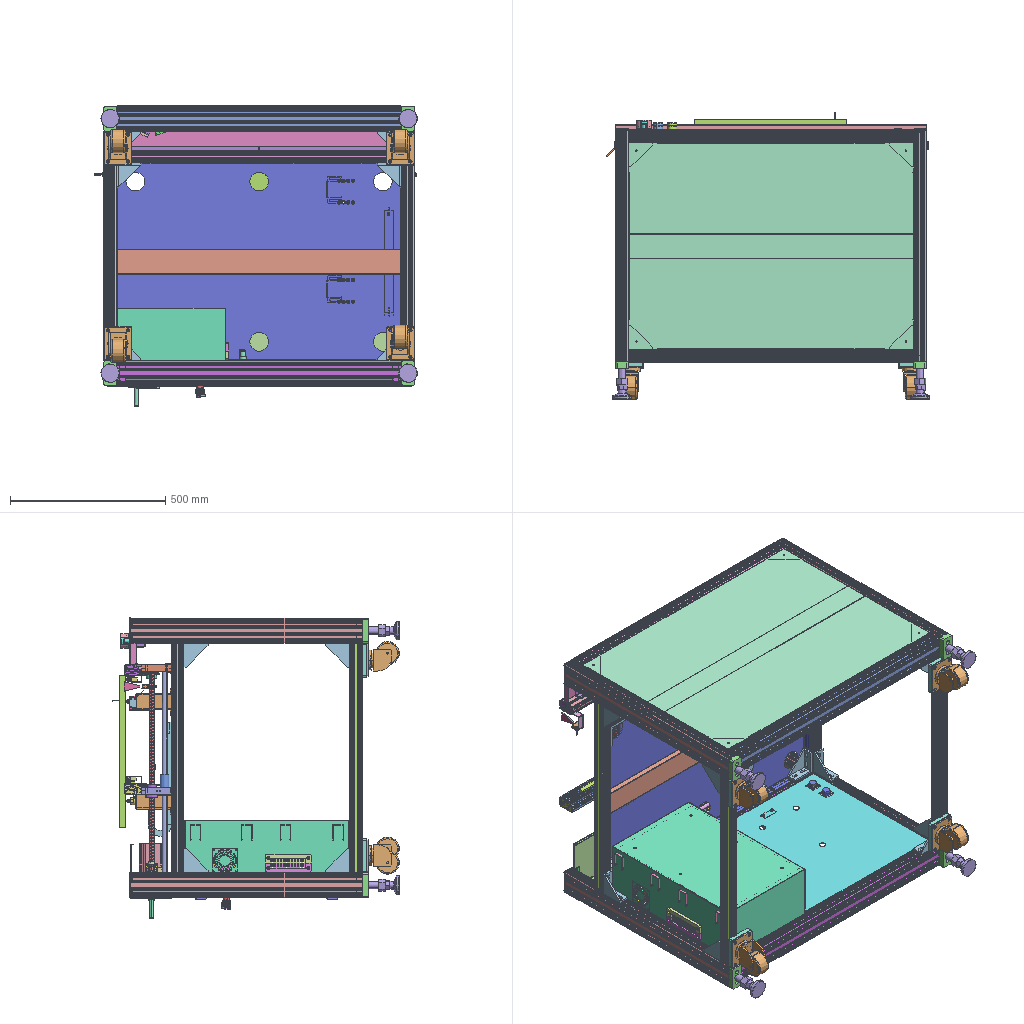Assembly | STEP file | 129 different items | 293 placed | box 1040 x 923 x 967 mm
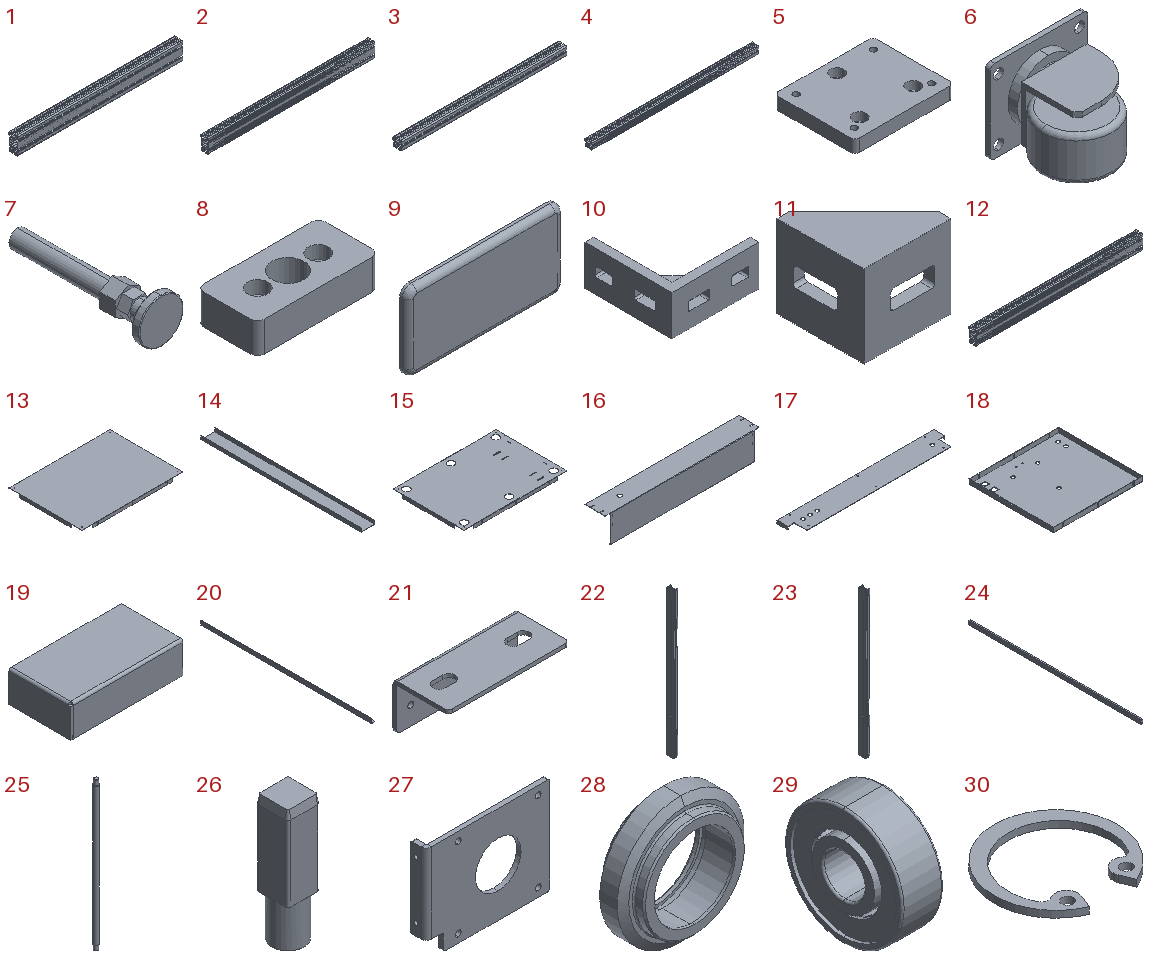Parts list (item | name | quantity | parent item | size | volume):
1 | MK-8-4080H-L-02 Profile 4080H Standard 747mm | x4 | in Transfer Station Profile Assembly | 747 x 40 x 80 mm | 606353 mm3
2 | MK-8-4080H-L-00 Profile 4080H Standard 920mm | x1 | in Transfer Station Profile Assembly | 920 x 40 x 80 mm | 746832 mm3
3 | MK-8-4040C-L-00 Profile 4040C Standard 740mm | x4 | in Transfer Station Profile Assembly | 740 x 40 x 40 mm | 353904 mm3
4 | MK-8-4040C-L-00 Profile 4040C Standard 920mm | x2 | in Transfer Station Profile Assembly | 920 x 40 x 40 mm | 439989 mm3
5 | - | x4 | in Transfer Station Profile Assembly | 110 x 90 x 14 mm | 130540 mm3
6 | 3-inch Heavy-Duty Caster 7223-222B | x4 | in Transfer Station Profile Assembly | 112 x 105 x 88 mm | 158459 mm3
7 | Carbon Steel Universal Leveling Foot KCUF M24-150-60 | x4 | in Transfer Station Profile Assembly | 60 x 195 x 60 mm | 136685 mm3
8 | Foot Mounting Block | x4 | in Transfer Station Profile Assembly | 80 x 40 x 20 mm | 52813 mm3
9 | End Cover Panel MK-EC-B-4080x4.3 | x4 | in Transfer Station Profile Assembly | 80 x 12.5 x 40 mm | 10356 mm3
10 | Die-cast Aluminum Connector, 40 Series, 40mm Face, Reinforced Type | x20 | in Transfer Station Profile Assembly | 78 x 78 x 36 mm | 52626 mm3
11 | Die-cast Aluminum Connector, 40 Series, 40mm Face, Standard Type | x2 | in Transfer Station Profile Assembly | 38 x 38 x 36 mm | 14409 mm3
12 | Aluminum Profile | x2 | in Transfer Station Profile Assembly | 920 x 40 x 80 mm | 738290 mm3
13 | Front Sheet Metal Cover Plate | x1 | - | 918 x 665 x 30 mm | 1014698 mm3
14 | - | x2 | - | 80 x 913 x 20 mm | 158644 mm3
15 | - | x1 | - | 918 x 636.5 x 30 mm | 1267450 mm3
16 | Rear Sheet Metal Cover Plate | x1 | - | 980 x 132 x 174.1 mm | 597177 mm3
17 | Button Mounting Plate | x1 | - | 1000 x 149 x 20 mm | 285929 mm3
18 | - | x1 | - | 566 x 533 x 32 mm | 714825 mm3
19 | - | x1 | - | 100 x 55 x 28 mm | 18799 mm3
20 | - | x1 | - | 20 x 900 x 23.6 mm | 73815 mm3
21 | Cover Plate Adapter Plate | x2 | - | 65 x 30 x 25 mm | 6480 mm3
22 | PN_0001 Line Front Chain Guide Channel L1000 | x1 | in Manual Width-Adjust Low-Precision Conveyor Line | 35 x 55 x 1000 mm | 771293 mm3
23 | PN_0001 Line Rear Chain Guide Channel L1000 | x1 | in Manual Width-Adjust Low-Precision Conveyor Line | 35 x 55 x 1000 mm | 771293 mm3
24 | PN_0001 06B Side Guide Chain Support Block L860 | x2 | in Manual Width-Adjust Low-Precision Conveyor Line | 9 x 860 x 20.4 mm | 137278 mm3
25 | - | x1 | in Manual Width-Adjust Low-Precision Conveyor Line | 15 x 15 x 460 mm | 78936 mm3
26 | PN_0001 Rotating Shaft Adapter Block | x1 | in Manual Width-Adjust Low-Precision Conveyor Line | 11.5 x 11.5 x 45 mm | 4695 mm3
27 | PN_0001 Tensioning Plate | x1 | in Manual Width-Adjust Low-Precision Conveyor Line | 108 x 14 x 85 mm | 32885 mm3
28 | - | x4 | - | 25 x 8.5 x 25 mm | 1521 mm3
29 | Deep Groove Ball Bearing 606-ZZ | x8 | - | 6 x 17 x 17 mm | 776.566 mm3
30 | PN_0002 Internal Retaining Ring Type A 17 | x8 | - | 18.3 x 17.603 x 1 mm | 85.781 mm3
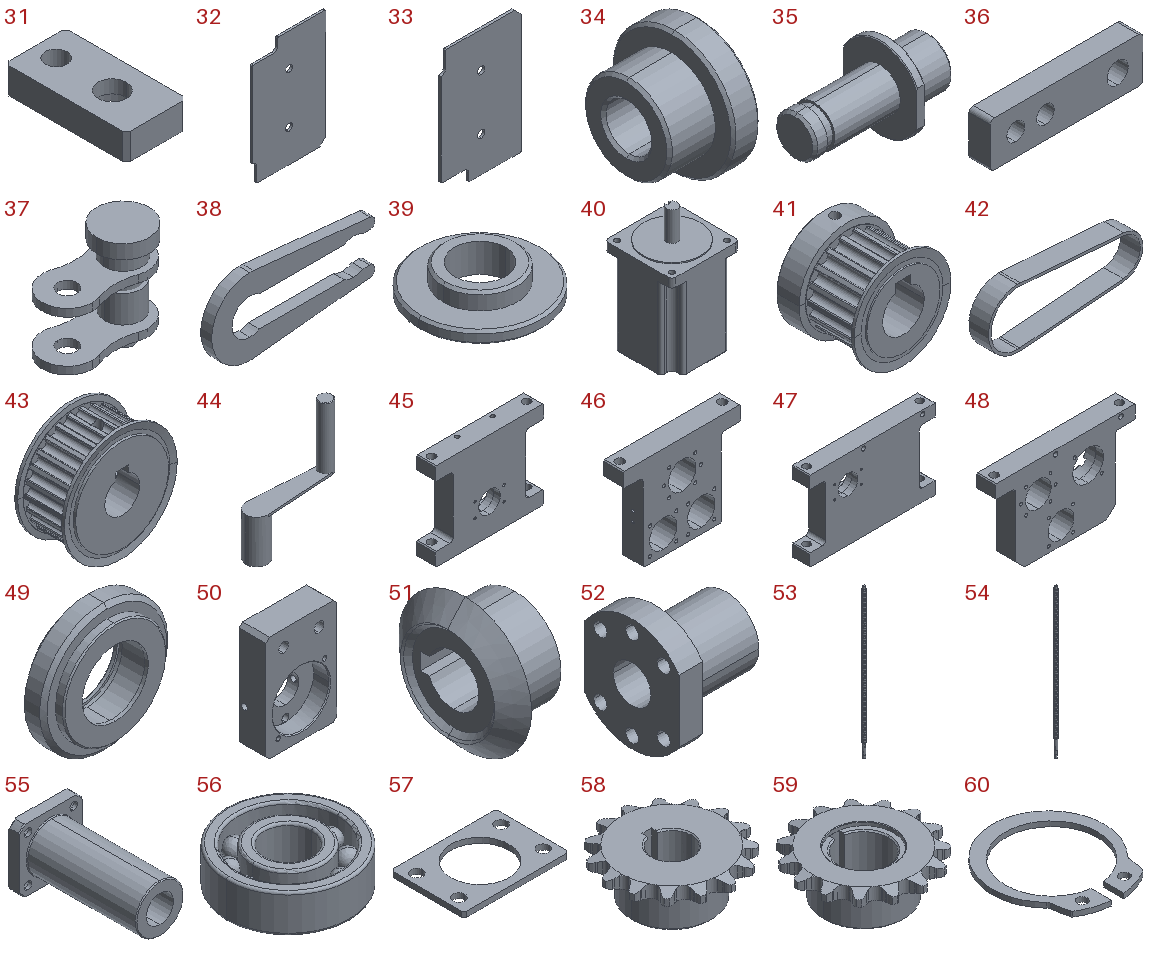31 | Front Guide Wheel Fixing Plate | x4 | in Manual Width-Adjust Low-Precision Conveyor Line | 14 x 28 x 6 mm | 1838 mm3
32 | Guide Channel Right End Cap | x2 | in Manual Width-Adjust Low-Precision Conveyor Line | 34.8 x 1 x 54.8 mm | 1804 mm3
33 | Guide Channel Left End Cap | x2 | in Manual Width-Adjust Low-Precision Conveyor Line | 34.8 x 1 x 54.8 mm | 1804 mm3
34 | Transition Guide Wheel | x4 | in Manual Width-Adjust Low-Precision Conveyor Line | 8 x 13.5 x 13.5 mm | 617.031 mm3
35 | Transition Guide Wheel Axle | x4 | in Manual Width-Adjust Low-Precision Conveyor Line | 16.4 x 9 x 10 mm | 405.919 mm3
36 | Driven Guide Wheel Connector | x4 | in Manual Width-Adjust Low-Precision Conveyor Line | 36 x 5 x 10.6 mm | 1667 mm3
37 | 06B Side Guide Chain | x2 | in Manual Width-Adjust Low-Precision Conveyor Line | 18.325 x 9 x 17.4 mm | 854.513 mm3
38 | 06B Side Guide Chain Buckle | x1 | in Manual Width-Adjust Low-Precision Conveyor Line | 15 x 1 x 7 mm | 49.292 mm3
39 | PN_0001 25 Small Sprocket Spacer Post | x4 | in Manual Width-Adjust Low-Precision Conveyor Line | 15 x 15 x 3.5 mm | 281.21 mm3
40 | Stepper Motor 34HS4801D14PJ5 | x1 | in Manual Width-Adjust Low-Precision Conveyor Line | 86 x 89 x 152.5 mm | 773985 mm3
41 | - | x1 | in Manual Width-Adjust Low-Precision Conveyor Line | 32.58 x 27 x 32.58 mm | 11988 mm3
42 | Timing Belt 270-5M-15mm Wide | x1 | in Manual Width-Adjust Low-Precision Conveyor Line | 119.02 x 15 x 45.38 mm | 8304 mm3
43 | - | x1 | in Manual Width-Adjust Low-Precision Conveyor Line | 45.32 x 21 x 45.32 mm | 21338 mm3
44 | Z-type Silver Iron Handle | x1 | in Manual Width-Adjust Low-Precision Conveyor Line | 80 x 20 x 97 mm | 17986 mm3
45 | PN_0001 Front Guide Channel Support Plate Left | x1 | in PN_0001 Lead Screw Type Adjusting Block Assembly | 120 x 21 x 97 mm | 164899 mm3
46 | Left Moving Support Plate | x1 | in PN_0001 Lead Screw Type Adjusting Block Assembly | 120 x 21 x 95 mm | 128293 mm3
47 | Front Guide Channel Support Plate Right | x1 | in PN_0001 Lead Screw Type Adjusting Block Assembly | 154 x 21 x 97 mm | 228293 mm3
48 | Right Moving Support Plate | x1 | in PN_0001 Lead Screw Type Adjusting Block Assembly | 154 x 21 x 95 mm | 178723 mm3
49 | - | x4 | - | 31 x 9 x 31 mm | 3611 mm3
50 | Drive Shaft Bearing Housing | x1 | in PN_0001 Lead Screw Type Adjusting Block Assembly | 40 x 15 x 59.5 mm | 24876 mm3
51 | KGKS1.0-3030-12 Bevel Gear | x4 | in PN_0001 Lead Screw Type Adjusting Block Assembly | - | -
52 | Nut SFU01604-4 | x2 | in Screw Pair SFUL1605-696, Handwheel Screw Pair SFUR1605-716 | 40 x 40 x 48 mm | 25660 mm3
53 | Screw SFUL1605-696 | x1 | in Screw Pair SFUL1605-696 | 16 x 16 x 696 mm | 120509 mm3
54 | Handwheel Screw SFUR1605-716 | x1 | in Handwheel Screw Pair SFUR1605-716 | 16 x 16 x 716 mm | 121693 mm3
55 | Bearing LMK16LUU | x3 | in PN_0001 Lead Screw Type Adjusting Block Assembly | 37 x 70 x 37 mm | 32483 mm3
56 | Bearing 6000Z_P5_BONA_ECO | x4 | in PN_0001 Lead Screw Type Adjusting Block Assembly | 26 x 26 x 8 mm | 2544 mm3
57 | 6001Z Bearing Stop Plate | x4 | in PN_0001 Lead Screw Type Adjusting Block Assembly | 40 x 28 x 2 mm | 1349 mm3
58 | - | x1 | in PN_0001 Lead Screw Type Adjusting Block Assembly | 50.395 x 50.132 x 19 mm | 15455 mm3
59 | - | x1 | in PN_0001 Lead Screw Type Adjusting Block Assembly | 50.395 x 50.132 x 19.5 mm | 13040 mm3
60 | Shaft Retaining Ring Type A 20 | x1 | in PN_0001 Lead Screw Type Adjusting Block Assembly | 22.5 x 25.161 x 1 mm | 155.824 mm3
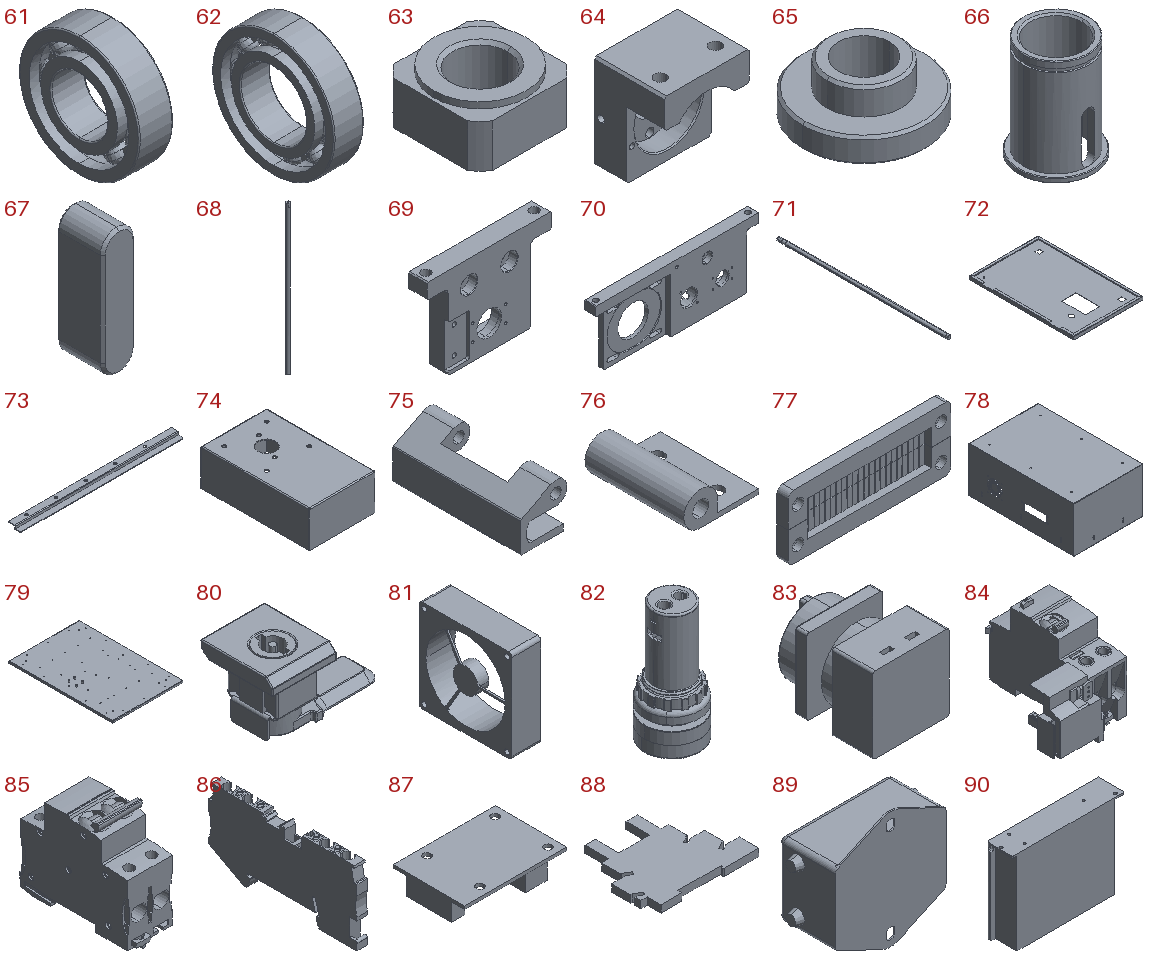61 | Bearing 6002Z | x4 | in PN_0001 Lead Screw Type Adjusting Block Assembly | 9 x 32 x 32 mm | 3871 mm3
62 | Bearing 6904Z | x1 | in PN_0001 Lead Screw Type Adjusting Block Assembly | 9 x 37 x 37 mm | 4601 mm3
63 | Lead Screw Support Block Lock Nut RN10 | x2 | in PN_0001 Lead Screw Type Adjusting Block Assembly | 16 x 16 x 8 mm | 1375 mm3
64 | PN_0001 Drive Bearing Housing | x1 | in PN_0001 Lead Screw Type Adjusting Block Assembly | 40 x 33 x 44.5 mm | 24608 mm3
65 | Sprocket Spacer Post | x4 | in PN_0001 Lead Screw Type Adjusting Block Assembly | 15 x 15 x 6.2 mm | 541.108 mm3
66 | Drive Shaft Sleeve | x1 | in PN_0001 Lead Screw Type Adjusting Block Assembly | 23 x 23 x 31.4 mm | 3535 mm3
67 | Key | x1 | in PN_0001 Lead Screw Type Adjusting Block Assembly | 3.9 x 5.5 x 15 mm | 300.753 mm3
68 | Support Shaft | x3 | in PN_0001 Lead Screw Type Adjusting Block Assembly | 16 x 16 x 680 mm | 136250 mm3
69 | PN_0001 Lead Screw Support Block Left | x1 | in PN_0001 Lead Screw Type Adjusting Block Assembly | 120 x 18 x 88 mm | 113336 mm3
70 | PN_0001 Lead Screw Support Block (Right) | x1 | in PN_0001 Lead Screw Type Adjusting Block Assembly | 268 x 18 x 105 mm | 283725 mm3
71 | PN_0001 Driving Shaft | x1 | in PN_0001 Lead Screw Type Adjusting Block Assembly | 16 x 710 x 16 mm | 135949 mm3
72 | - | x2 | - | 350 x 530 x 17 mm | 262811 mm3
73 | Cover Reinforcing Rib 275mm | x2 | - | 275 x 21 x 6 mm | 6947 mm3
74 | Power Knob Mounting Sheet Metal | x2 | - | 74 x 122 x 41 mm | 24069 mm3
75 | Hinge CL237Z3H001-01 | x4 | in Hinge CL237Z3H001 | 17.5 x 48 x 18 mm | 5234 mm3
76 | Hinge CL237Z3H001-02 | x4 | in Hinge CL237Z3H001 | 19 x 25 x 8.5 mm | 1495 mm3
77 | Cabinet Brush KEL-BES-S24 | x2 | - | 148 x 10 x 58 mm | 60298 mm3
78 | Electrical Cabinet Base | x2 | - | 350 x 530 x 243.8 mm | 759482 mm3
79 | - | x2 | - | 335 x 495 x 18 mm | 269254 mm3
80 | Cylinder Lock MS813-Shengjiu | x2 | - | 58.793 x 35 x 31.6 mm | 16415 mm3
81 | Axial Fan RDH8025B2_24V DC_3000RPM_ECO | x1 | - | 25 x 80 x 80 mm | 69901 mm3
82 | Indicator Light AD17-22-AC220VW White | x1 | - | 29 x 29.009 x 63.018 mm | 9405 mm3
83 | Power Switch LW42B2-1824_L | x1 | - | 65.5 x 92 x 65.5 mm | 250369 mm3
84 | Residual Current Device Vigi-iC65-ELE-2P-40A-30mA-A | x1 | - | 76.2 x 105.618 x 73.908 mm | 172404 mm3
85 | Miniature Circuit Breaker IC65N-2P-C16A | x1 | - | 35.4 x 93.9 x 74.3 mm | 159125 mm3
86 | Feed-through Terminal Block PT2,5-QUATTRO-3209578 | x18 | - | 5.15 x 72.2 x 35.25 mm | 9561 mm3
87 | LJ1XH6-2EDGK Circuit Board Assembly | x1 | - | 54 x 38 x 11.5 mm | 8666 mm3
88 | Miniature Medium-Power Relay HF41F_24-ZST and Socket 41F-1Z-C2-1 | x2 | - | 88 x 75.5 x 6.1 mm | 25363 mm3
89 | Power Filter CA5-W43B | x1 | - | 53.2 x 24 x 50 mm | 35444 mm3
90 | Switching Power Supply LRS-100-24 | x1 | - | 129 x 30 x 97 mm | 340596 mm3
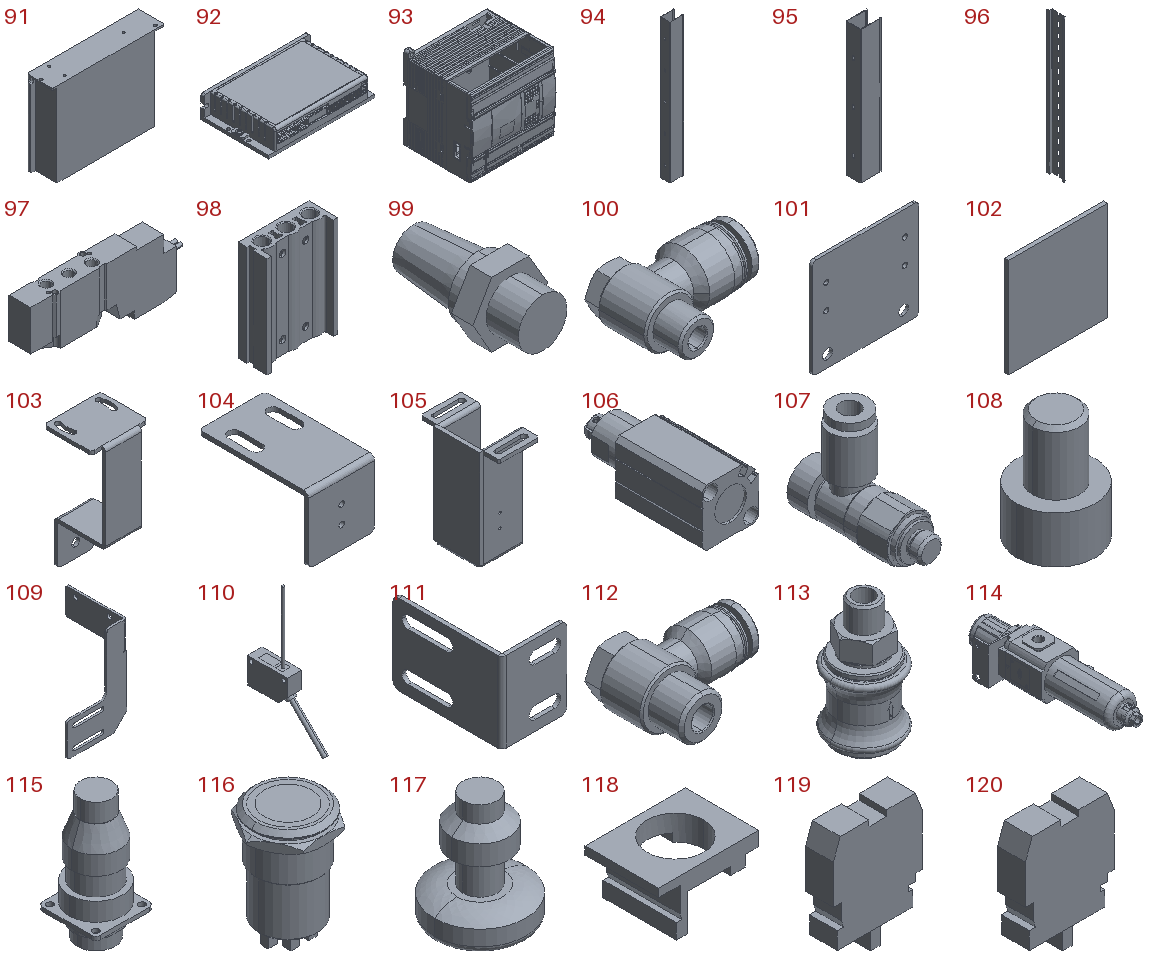91 | Switching Power Supply LRS-100-48 | x1 | - | 129 x 30 x 97 mm | 340596 mm3
92 | Stepper Motor Driver DM542-KK V3.0 | x1 | - | 119 x 77.6 x 25.5 mm | 99944 mm3
93 | Programmable Controller XD3-32T-E | x1 | - | - | -
94 | 35 Cable Tray_508 | x2 | - | 50.625 x 35 x 508 mm | 68787 mm3
95 | 35 Cable Tray_314 | x4 | - | 50.625 x 35 x 314 mm | 42522 mm3
96 | - | x2 | - | 5.5 x 35 x 280 mm | 5866 mm3
97 | 5-Port Solenoid Valve SY3120-5G-M5 | x2 | - | 72.9 x 11.6 x 28.5 mm | 14643 mm3
98 | Solenoid Valve Manifold SS5Y3-20-04_Default | x1 | - | 49 x 20 x 69.5 mm | 33276 mm3
99 | Universal Copper Muffler BSL-01 | x4 | - | 13.856 x 24 x 12 mm | 1771 mm3
100 | Hex Shaft Joint APH8-01 | x1 | - | 33.351 x 25 x 15 mm | 4443 mm3
101 | Solenoid Valve Mounting Adapter Plate | x1 | - | 70 x 2 x 65 mm | 8883 mm3
102 | - | x1 | - | 490 x 20 x 490 mm | 4802000 mm3
103 | - | x3 | - | 33 x 38 x 75 mm | 6071 mm3
104 | - | x1 | - | 30 x 50 x 30 mm | 4308 mm3
105 | - | x2 | in Stopper Assembly | 49.01 x 88 x 115 mm | 72509 mm3
106 | Stopper Cylinder TWQ-S-20x10-R | x2 | in Stopper Assembly | - | -
107 | Speed Control Valve AS1201F-M5-04A | x4 | in Stopper Assembly | 9.373 x 25.4 x 22 mm | 1869 mm3
108 | M6X8 Hex Socket Screw | x1 | in Stopper Assembly | 10 x 10 x 14 mm | 616.111 mm3
109 | Sensor Mounting Plate | x1 | - | 45 x 45 x 70 mm | 3643 mm3
110 | Miniature Photoelectric Sensor CX-441 | x1 | - | 11.2 x 58.715 x 100.215 mm | 7246 mm3
111 | Stop Mounting Plate | x2 | - | 34 x 57 x 42 mm | 6375 mm3
112 | Hex Shaft Joint APH8-02 | x1 | - | 37.183 x 28 x 17.166 mm | 6274 mm3
113 | Hand Slide Valve HSV08 | x1 | - | - | -
114 | Pressure Regulating Filter GFR300-08-N | x1 | - | - | -
115 | SMEMA Connector | x2 | - | 36 x 36 x 78.52 mm | 45655 mm3
116 | Metal Push Button Switch Ring Light GQ22-L-11E_G_24V_S | x2 | - | 28.5 x 25 x 38.7 mm | 12469 mm3
117 | - | x1 | - | 40 x 40 x 48 mm | 24355 mm3
118 | Connecting Bracket LA42-PT-ZJ | x3 | - | 41 x 30 x 22 mm | 6377 mm3
119 | Contact Block LA42-01-NC | x3 | - | 32 x 10 x 42 mm | 10410 mm3
120 | Contact Block LA42-10-NO | x3 | - | 32 x 10 x 42 mm | 10410 mm3
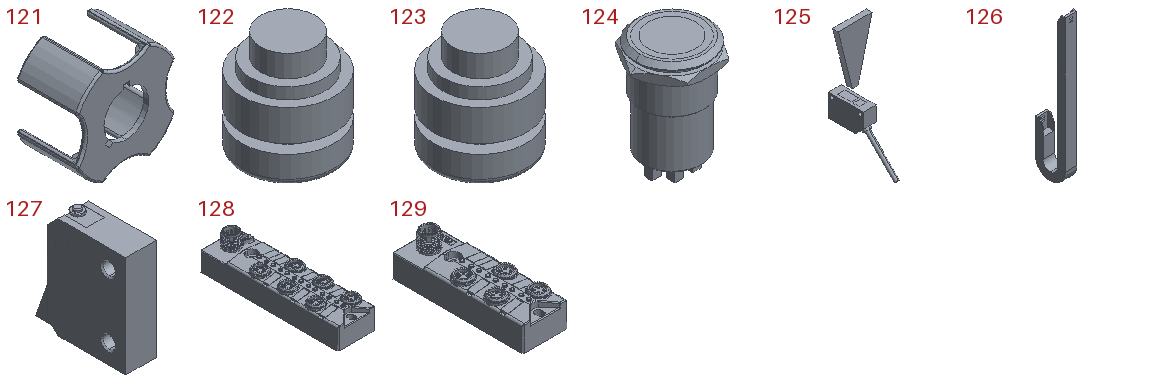121 | Emergency Stop Guard Ring J-V | x1 | - | 47.915 x 30.4 x 47.915 mm | 9284 mm3
122 | - | x1 | - | 30 x 30 x 33 mm | 18043 mm3
123 | Button Head LA42PD-G | x1 | - | 30 x 30 x 33 mm | 18043 mm3
124 | Metal Push Button Switch Ring Light GQ22-L-11E_Y_24V_S | x1 | - | 28.5 x 25 x 38.7 mm | 12469 mm3
125 | Limited Reflective Photoelectric Switch CX-462A | x3 | - | 30 x 58.715 x 105.315 mm | 11448 mm3
126 | Cable Carrier J15BF.1.20N28 | x1 | - | 28.5 x 74.5 x 367.25 mm | 251972 mm3
127 | Stopper Assembly PFC01-7SA-R-MK | x2 | - | 12 x 38 x 42 mm | 13788 mm3
128 | I/O Junction Box 23N6S1 | x1 | - | - | -
129 | I/O Junction Box 23N4S1 | x1 | - | 29.939 x 86.939 x 25.75 mm | 38975 mm3
Placements (level | parent | child | x y z in mm | rotation matrix by rows), first 215 of 321 lines:
1 | subassembly 2 | Transfer Station Frame Assembly | -191.936 1251.56 494.518 | 1 0 0 0 1 0 0 0 1
2 | Transfer Station Frame Assembly | Transfer Station Profile Assembly | 742.606 -805.957 -90.772 | 1 0 0 0 1 0 0 0 1
3 | Transfer Station Profile Assembly | MK-8-4080H-L-02 Profile 4080H Standard 747mm | -2740.268 -854.394 110.646 | 0 1 0 1 0 0 0 0 -1
3 | Transfer Station Profile Assembly | MK-8-4080H-L-00 Profile 4080H Standard 920mm | -2720.268 -834.394 110.646 | 1 0 0 0 -1 0 0 0 -1
3 | Transfer Station Profile Assembly | MK-8-4040C-L-00 Profile 4040C Standard 740mm | -2740.268 -834.394 70.646 | 0 1 0 0 0 -1 -1 0 -0
3 | Transfer Station Profile Assembly | MK-8-4040C-L-00 Profile 4040C Standard 740mm | -1780.268 -834.394 70.646 | 0 1 0 0 0 -1 -1 0 -0
3 | Transfer Station Profile Assembly | MK-8-4040C-L-00 Profile 4040C Standard 920mm | -2720.268 -127.394 130.646 | 1 0 0 0 1 0 0 0 1
3 | Transfer Station Profile Assembly | MK-8-4040C-L-00 Profile 4040C Standard 920mm | -2720.268 -259.394 -10.854 | 1 0 0 0 1 0 0 0 1
3 | Transfer Station Profile Assembly | subassembly 3 | -1805.268 -854.394 -614.354 | 0 -1 0 0 0 -1 1 0 -0
3 | Transfer Station Profile Assembly | subassembly 3 | -1805.268 -854.394 15.646 | 0 -1 0 0 0 -1 1 0 -0
3 | Transfer Station Profile Assembly | 3-inch Heavy-Duty Caster 7223-222B | -1805.268 -873.394 -614.354 | 0 0 1 0 1 0 -1 0 0
3 | Transfer Station Profile Assembly | 3-inch Heavy-Duty Caster 7223-222B | -1805.268 -873.394 15.646 | 0 0 1 0 1 0 -1 0 0
3 | Transfer Station Profile Assembly | Carbon Steel Universal Leveling Foot KCUF M24-150-60 | -1780.268 -973.394 -709.354 | 0.6285 0 0.7778 0 1 0 -0.7778 0 0.6285
3 | Transfer Station Profile Assembly | Carbon Steel Universal Leveling Foot KCUF M24-150-60 | -1780.268 -973.394 110.646 | 0.6285 0 0.7778 0 1 0 -0.7778 0 0.6285
3 | Transfer Station Profile Assembly | Foot Mounting Block | -1780.268 -854.394 -709.354 | 0 1 0 0 0 -1 -1 0 -0
3 | Transfer Station Profile Assembly | Foot Mounting Block | -1780.268 -854.394 110.646 | 0 1 0 0 0 -1 -1 0 -0
3 | Transfer Station Profile Assembly | End Cover Panel MK-EC-B-4080x4.3 | -2740.268 -103.094 110.646 | 0 0 1 0 -1 0 1 0 0
3 | Transfer Station Profile Assembly | Die-cast Aluminum Connector, 40 Series, 40mm Face, Reinforced Type | -2720.268 -852.394 -669.354 | 0 1 0 0 0 1 1 0 0
3 | Transfer Station Profile Assembly | Die-cast Aluminum Connector, 40 Series, 40mm Face, Reinforced Type | -2720.268 -852.394 70.646 | 1 0 0 0 0 1 0 -1 0
3 | Transfer Station Profile Assembly | Die-cast Aluminum Connector, 40 Series, 40mm Face, Reinforced Type | -1800.268 -852.394 -669.354 | -1 0 0 0 0 1 0 1 0
3 | Transfer Station Profile Assembly | Die-cast Aluminum Connector, 40 Series, 40mm Face, Reinforced Type | -1800.268 -852.394 70.646 | 0 -1 0 0 0 1 -1 0 0
3 | Transfer Station Profile Assembly | Die-cast Aluminum Connector, 40 Series, 40mm Face, Reinforced Type | -2720.268 -814.394 148.646 | 0 1 0 1 0 0 0 0 -1
3 | Transfer Station Profile Assembly | Die-cast Aluminum Connector, 40 Series, 40mm Face, Reinforced Type | -1800.268 -814.394 148.646 | -1 0 0 0 1 0 0 0 -1
3 | Transfer Station Profile Assembly | Die-cast Aluminum Connector, 40 Series, 40mm Face, Reinforced Type | -1800.268 -147.394 148.646 | 0 -1 0 -1 0 0 0 0 -1
3 | Transfer Station Profile Assembly | Die-cast Aluminum Connector, 40 Series, 40mm Face, Reinforced Type | -2720.268 -147.394 148.646 | 1 0 0 0 -1 0 0 0 -1
3 | Transfer Station Profile Assembly | Die-cast Aluminum Connector, 40 Series, 40mm Face, Reinforced Type | -2758.268 -814.394 -669.354 | 0 0 1 1 0 0 0 1 0
3 | Transfer Station Profile Assembly | Die-cast Aluminum Connector, 40 Series, 40mm Face, Reinforced Type | -2758.268 -814.394 70.646 | 0 0 1 0 1 0 -1 0 0
3 | Transfer Station Profile Assembly | Die-cast Aluminum Connector, 40 Series, 40mm Face, Reinforced Type | -2758.268 -279.394 70.646 | 0 0 1 -1 0 0 0 -1 0
3 | Transfer Station Profile Assembly | Die-cast Aluminum Connector, 40 Series, 40mm Face, Reinforced Type | -2758.268 -279.394 -669.354 | 0 0 1 0 -1 0 1 0 0
3 | Transfer Station Profile Assembly | Die-cast Aluminum Connector, 40 Series, 40mm Face, Reinforced Type | -1800.268 -241.394 -30.854 | -1 0 0 0 0 -1 0 -1 -0
3 | Transfer Station Profile Assembly | Die-cast Aluminum Connector, 40 Series, 40mm Face, Reinforced Type | -2720.268 -241.394 -30.854 | 0 1 0 0 0 -1 -1 0 -0
3 | Transfer Station Profile Assembly | Die-cast Aluminum Connector, 40 Series, 40mm Face, Reinforced Type | -1800.268 -241.394 -669.354 | 0 -1 0 0 0 -1 1 0 -0
3 | Transfer Station Profile Assembly | Die-cast Aluminum Connector, 40 Series, 40mm Face, Reinforced Type | -2720.268 -241.394 -669.354 | 1 0 0 0 0 -1 0 1 -0
3 | Transfer Station Profile Assembly | Die-cast Aluminum Connector, 40 Series, 40mm Face, Standard Type | -1800.268 -259.394 9.146 | 0 -1 0 0 0 -1 1 0 -0
3 | Transfer Station Profile Assembly | Die-cast Aluminum Connector, 40 Series, 40mm Face, Standard Type | -2720.268 -259.394 9.146 | 1 0 0 0 0 -1 0 1 -0
3 | Transfer Station Profile Assembly | 3-inch Heavy-Duty Caster 7223-222B | -2715.268 -873.394 15.646 | 0 0 1 0 1 0 -1 0 0
3 | Transfer Station Profile Assembly | subassembly 3 | -2715.268 -854.394 15.646 | 0 1 0 0 0 -1 -1 0 0
3 | Transfer Station Profile Assembly | 3-inch Heavy-Duty Caster 7223-222B | -2715.268 -873.394 -614.354 | 0 0 -1 0 1 0 1 0 -0
3 | Transfer Station Profile Assembly | subassembly 3 | -2715.268 -854.394 -614.354 | 0 1 0 0 0 -1 -1 0 -0
3 | Transfer Station Profile Assembly | MK-8-4080H-L-02 Profile 4080H Standard 747mm | -2740.268 -854.394 -709.354 | 0 1 0 1 0 0 0 0 -1
3 | Transfer Station Profile Assembly | MK-8-4080H-L-02 Profile 4080H Standard 747mm | -1780.268 -854.394 110.646 | 0 1 0 1 0 0 0 0 -1
3 | Transfer Station Profile Assembly | MK-8-4080H-L-02 Profile 4080H Standard 747mm | -1780.268 -854.394 -709.354 | 0 1 0 1 0 0 0 0 -1
3 | Transfer Station Profile Assembly | Aluminum Profile | -2720.268 -259.394 -709.354 | 1 0 0 0 -1 0 0 0 -1
3 | Transfer Station Profile Assembly | Aluminum Profile | -2720.268 -834.394 -709.354 | 1 0 0 0 -1 0 0 0 -1
3 | Transfer Station Profile Assembly | MK-8-4040C-L-00 Profile 4040C Standard 740mm | -1780.268 -259.394 70.646 | 0 1 0 0 0 -1 -1 0 -0
3 | Transfer Station Profile Assembly | MK-8-4040C-L-00 Profile 4040C Standard 740mm | -2740.268 -259.394 70.646 | 0 1 0 0 0 -1 -1 0 -0
3 | Transfer Station Profile Assembly | End Cover Panel MK-EC-B-4080x4.3 | -1780.268 -103.094 110.646 | 0 0 1 0 -1 0 1 0 0
3 | Transfer Station Profile Assembly | End Cover Panel MK-EC-B-4080x4.3 | -2740.268 -103.094 -709.354 | 0 0 1 0 -1 0 1 0 0
3 | Transfer Station Profile Assembly | End Cover Panel MK-EC-B-4080x4.3 | -1780.268 -103.094 -709.354 | 0 0 1 0 -1 0 1 0 0
3 | Transfer Station Profile Assembly | Carbon Steel Universal Leveling Foot KCUF M24-150-60 | -2740.268 -973.394 110.646 | 0.6285 0 0.7778 0 1 0 -0.7778 0 0.6285
3 | Transfer Station Profile Assembly | Foot Mounting Block | -2740.268 -854.394 110.646 | 0 1 0 0 0 -1 -1 0 -0
3 | Transfer Station Profile Assembly | Carbon Steel Universal Leveling Foot KCUF M24-150-60 | -2740.268 -973.394 -709.354 | 0.6285 0 0.7778 0 1 0 -0.7778 0 0.6285
3 | Transfer Station Profile Assembly | Foot Mounting Block | -2740.268 -854.394 -709.354 | 0 1 0 0 0 -1 -1 0 -0
3 | Transfer Station Profile Assembly | Die-cast Aluminum Connector, 40 Series, 40mm Face, Reinforced Type | -1798.268 -279.394 70.646 | 0 0 1 -1 0 0 0 -1 0
3 | Transfer Station Profile Assembly | Die-cast Aluminum Connector, 40 Series, 40mm Face, Reinforced Type | -1798.268 -814.394 70.646 | 0 0 1 0 1 0 -1 0 0
3 | Transfer Station Profile Assembly | Die-cast Aluminum Connector, 40 Series, 40mm Face, Reinforced Type | -1798.268 -814.394 -669.354 | 0 0 1 1 0 0 0 1 0
3 | Transfer Station Profile Assembly | Die-cast Aluminum Connector, 40 Series, 40mm Face, Reinforced Type | -1798.268 -279.394 -669.354 | 0 0 1 0 -1 0 1 0 0
2 | Transfer Station Frame Assembly | subassembly 4 | -1697.809 -1807.536 -612.222 | 1 0 0 0 1 0 0 0 1
3 | subassembly 4 | Front Sheet Metal Cover Plate | 180.147 520.685 671.596 | 1 0 0 0 1 0 0 0 1
3 | subassembly 4 | subassembly 5 | 180.147 480.685 650.096 | 0 -1 0 1 0 0 0 0 1
2 | Transfer Station Frame Assembly | subassembly 6 | -1727.029 -1794.632 98.097 | 1 0 0 0 0 1 0 -1 0
3 | subassembly 6 | subassembly 7 | 209.367 538.973 749.281 | 1 0 0 0 1 0 0 0 1
3 | subassembly 6 | subassembly 5 | 209.367 498.973 727.281 | 0 -1 0 1 0 0 0 0 1
1 | subassembly 2 | Rear Sheet Metal Cover Plate | -1709.598 336.209 -259.508 | 1 0 0 0 -1 0 0 0 -1
1 | subassembly 2 | Button Mounting Plate | -1709.598 340.209 406.392 | 1 0 0 0 0 1 0 -1 0
1 | subassembly 2 | subassembly 8 | -1546.601 -61.664 -299.141 | 1 0 0 0 1 0 0 0 1
2 | subassembly 8 | subassembly 9 | 14.002 -39.627 31.533 | -1 0 0 0 1 0 0 0 -1
2 | subassembly 8 | subassembly 10 | -216.998 -39.627 3.533 | -1 0 0 0 1 0 0 0 -1
1 | subassembly 2 | subassembly 11 | -1709.598 338.209 405.392 | 0 -1 0 0 0 -1 1 0 0
1 | subassembly 2 | Cover Plate Adapter Plate | -1249.598 321.209 -305.608 | 0 0 1 0 1 0 -1 0 0
1 | subassembly 2 | Cover Plate Adapter Plate | -2169.598 321.209 -305.608 | 0 0 -1 0 1 0 1 0 -0
1 | subassembly 2 | Manual Width-Adjust Low-Precision Conveyor Line | -1762.856 197.208 792.663 | -1 0 0 0 1 0 0 0 -1
2 | Manual Width-Adjust Low-Precision Conveyor Line | PN_0001 Line Front Chain Guide Channel L1000 | -53.257 136.585 419.271 | 0 0 -1 0 1 0 1 0 -0
2 | Manual Width-Adjust Low-Precision Conveyor Line | PN_0001 Line Rear Chain Guide Channel L1000 | -53.257 136.585 772.708 | 0 0 1 0 1 0 -1 0 0
2 | Manual Width-Adjust Low-Precision Conveyor Line | PN_0001 06B Side Guide Chain Support Block L860 | -53.257 137.7 769.208 | 0 -1 0 0 0 -1 1 0 -0
2 | Manual Width-Adjust Low-Precision Conveyor Line | subassembly 12 | 35.743 73.0 1048.271 | 0 0 -1 0.1015 0.9948 0 0.9948 -0.1015 -0
2 | Manual Width-Adjust Low-Precision Conveyor Line | PN_0001 Rotating Shaft Adapter Block | 278.243 73.0 1092.271 | 1 0 0 0 1 0 0 0 1
2 | Manual Width-Adjust Low-Precision Conveyor Line | PN_0001 Tensioning Plate | -400.657 26.5 1084.771 | 1 0 0 0 0 1 0 -1 0
2 | Manual Width-Adjust Low-Precision Conveyor Line | PN_0001 06B Side Guide Chain Support Block L860 | -53.257 137.7 422.771 | 0 1 0 0 0 -1 -1 0 -0
2 | Manual Width-Adjust Low-Precision Conveyor Line | subassembly 13 | 375.815 133.424 747.736 | -0.2668 0 0.9637 0.9637 0 0.2668 0 1 0
3 | subassembly 13 | subassembly 14 | -6.597 27.473 34.415 | 1 0 0 0 1 0 0 0 1
3 | subassembly 13 | Deep Groove Ball Bearing 606-ZZ | -6.597 26.473 34.415 | 0 1 0 -1 0 0 0 0 1
3 | subassembly 13 | PN_0002 Internal Retaining Ring Type A 17 | -6.597 30.023 34.415 | 1 0 0 0 0 -1 0 1 0
2 | Manual Width-Adjust Low-Precision Conveyor Line | subassembly 13 | -482.159 154.193 444.244 | -0.3412 0 -0.94 0.94 0 -0.3412 0 -1 -0
3 | subassembly 13 | subassembly 14 | -6.597 27.473 34.415 | 1 0 0 0 1 0 0 0 1
3 | subassembly 13 | Deep Groove Ball Bearing 606-ZZ | -6.597 26.473 34.415 | 0 1 0 -1 0 0 0 0 1
3 | subassembly 13 | PN_0002 Internal Retaining Ring Type A 17 | -6.597 30.023 34.415 | 1 0 0 0 0 -1 0 1 0
2 | Manual Width-Adjust Low-Precision Conveyor Line | subassembly 13 | 398.466 170.527 444.244 | -0.9998 0 0.0198 -0.0198 0 -0.9998 0 -1 -0
3 | subassembly 13 | subassembly 14 | -6.597 27.473 34.415 | 1 0 0 0 1 0 0 0 1
3 | subassembly 13 | Deep Groove Ball Bearing 606-ZZ | -6.597 26.473 34.415 | 0 1 0 -1 0 0 0 0 1
3 | subassembly 13 | PN_0002 Internal Retaining Ring Type A 17 | -6.597 30.023 34.415 | 1 0 0 0 0 -1 0 1 0
2 | Manual Width-Adjust Low-Precision Conveyor Line | subassembly 13 | -521.696 101.491 747.736 | -0.9981 0 -0.06234 -0.06234 0 0.9981 0 1 0
3 | subassembly 13 | subassembly 14 | -6.597 27.473 34.415 | 1 0 0 0 1 0 0 0 1
3 | subassembly 13 | Deep Groove Ball Bearing 606-ZZ | -6.597 26.473 34.415 | 0 1 0 -1 0 0 0 0 1
3 | subassembly 13 | PN_0002 Internal Retaining Ring Type A 17 | -6.597 30.023 34.415 | 1 0 0 0 0 -1 0 1 0
2 | Manual Width-Adjust Low-Precision Conveyor Line | Front Guide Wheel Fixing Plate | -546.257 138.5 774.708 | 1 0 0 0 1 0 0 0 1
2 | Manual Width-Adjust Low-Precision Conveyor Line | Front Guide Wheel Fixing Plate | -546.257 138.5 417.271 | -1 0 0 0 1 0 0 0 -1
2 | Manual Width-Adjust Low-Precision Conveyor Line | Front Guide Wheel Fixing Plate | 439.743 138.5 417.271 | -1 0 0 0 1 0 0 0 -1
2 | Manual Width-Adjust Low-Precision Conveyor Line | Front Guide Wheel Fixing Plate | 439.743 138.5 774.708 | 1 0 0 0 1 0 0 0 1
2 | Manual Width-Adjust Low-Precision Conveyor Line | Guide Channel Right End Cap | -554.257 133.5 404.771 | 0 1 0 0 0 -1 -1 0 -0
2 | Manual Width-Adjust Low-Precision Conveyor Line | Guide Channel Right End Cap | 447.743 133.5 787.208 | 0 -1 0 0 0 -1 1 0 -0
2 | Manual Width-Adjust Low-Precision Conveyor Line | Guide Channel Left End Cap | 447.743 133.5 404.771 | 0 -1 0 0 0 1 -1 0 0
2 | Manual Width-Adjust Low-Precision Conveyor Line | Guide Channel Left End Cap | -554.257 133.5 787.208 | 0 1 0 0 0 1 1 0 0
2 | Manual Width-Adjust Low-Precision Conveyor Line | Transition Guide Wheel | -546.257 149.15 423.271 | 0 0.9998 -0.02004 0 0.02004 0.9998 1 0 0
2 | Manual Width-Adjust Low-Precision Conveyor Line | Transition Guide Wheel | 439.743 149.15 423.271 | 0 -0.09453 -0.9955 0 0.9955 -0.09453 1 0 -0
2 | Manual Width-Adjust Low-Precision Conveyor Line | Transition Guide Wheel | 439.743 149.15 768.708 | 0 -0.09453 0.9955 0 0.9955 0.09453 -1 0 0
2 | Manual Width-Adjust Low-Precision Conveyor Line | Transition Guide Wheel | -546.257 149.15 768.708 | 0 -0.09453 0.9955 0 0.9955 0.09453 -1 0 0
2 | Manual Width-Adjust Low-Precision Conveyor Line | Transition Guide Wheel Axle | -546.257 149.15 418.271 | 0 -0.09453 0.9955 0 0.9955 0.09453 -1 0 0
2 | Manual Width-Adjust Low-Precision Conveyor Line | Transition Guide Wheel Axle | 439.743 149.15 418.271 | 0 -0.09453 0.9955 0 0.9955 0.09453 -1 0 0
2 | Manual Width-Adjust Low-Precision Conveyor Line | Transition Guide Wheel Axle | -546.257 149.15 773.708 | 0 -0.09453 -0.9955 0 0.9955 -0.09453 1 0 -0
2 | Manual Width-Adjust Low-Precision Conveyor Line | Transition Guide Wheel Axle | 439.743 149.15 773.708 | 0 -0.8433 0.5374 0 -0.5374 -0.8433 1 0 -0
2 | Manual Width-Adjust Low-Precision Conveyor Line | Driven Guide Wheel Connector | -505.257 136.25 788.208 | -1 0 0 0 0 1 0 1 0
2 | Manual Width-Adjust Low-Precision Conveyor Line | Driven Guide Wheel Connector | -500.257 136.25 408.771 | -1 0 0 0 0 1 0 1 0
2 | Manual Width-Adjust Low-Precision Conveyor Line | Driven Guide Wheel Connector | 398.743 136.25 788.208 | 1 0 0 0 0 -1 0 1 -0
2 | Manual Width-Adjust Low-Precision Conveyor Line | Driven Guide Wheel Connector | 393.743 136.25 408.771 | 1 0 0 0 0 -1 0 1 -0
2 | Manual Width-Adjust Low-Precision Conveyor Line | 06B Side Guide Chain | -295.164 152.0 765.268 | -1 0 0 0 1 0 0 0 -1
2 | Manual Width-Adjust Low-Precision Conveyor Line | 06B Side Guide Chain | -295.164 152.0 406.831 | 0.9981 0.06163 0 0.06163 -0.9981 0 0 0 -1
2 | Manual Width-Adjust Low-Precision Conveyor Line | 06B Side Guide Chain Buckle | -290.423 152.45 769.268 | 0.9955 0 0.09453 0.09453 0 -0.9955 0 1 -0
2 | Manual Width-Adjust Low-Precision Conveyor Line | PN_0001 25 Small Sprocket Spacer Post | -517.257 136.25 780.708 | -0.8834 -0.4687 0 -0.4687 0.8834 0 0 0 -1
2 | Manual Width-Adjust Low-Precision Conveyor Line | PN_0001 25 Small Sprocket Spacer Post | -512.257 136.25 411.271 | 0.9955 -0.09453 0 0.09453 0.9955 0 0 0 1
2 | Manual Width-Adjust Low-Precision Conveyor Line | PN_0001 25 Small Sprocket Spacer Post | 405.743 136.25 411.271 | 0.9955 -0.09453 0 0.09453 0.9955 0 0 0 1
2 | Manual Width-Adjust Low-Precision Conveyor Line | PN_0001 25 Small Sprocket Spacer Post | 410.743 136.25 780.708 | -0.8834 -0.4687 0 -0.4687 0.8834 0 0 0 -1
2 | Manual Width-Adjust Low-Precision Conveyor Line | Stepper Motor 34HS4801D14PJ5 | -341.657 69.0 963.271 | 0 1 0 -1 0 0 0 0 1
2 | Manual Width-Adjust Low-Precision Conveyor Line | subassembly 15 | -341.657 69.0 1115.771 | 0.6077 0 -0.7941 -0.7941 0 -0.6077 0 1 -0
2 | Manual Width-Adjust Low-Precision Conveyor Line | Timing Belt 270-5M-15mm Wide | -261.757 73.0 1099.771 | -0.9987 0 -0.05 -0.05 0 0.9987 0 1 0
2 | Manual Width-Adjust Low-Precision Conveyor Line | subassembly 16 | -261.757 73.0 1098.771 | -0.1835 0 0.983 0.983 0 0.1835 0 1 0
2 | Manual Width-Adjust Low-Precision Conveyor Line | Z-type Silver Iron Handle | 278.243 73.0 1107.271 | 1 -0.007063 0 0.007063 1 0 0 0 1
2 | Manual Width-Adjust Low-Precision Conveyor Line | PN_0001 Lead Screw Type Adjusting Block Assembly | 278.243 58.5 731.771 | 1 0 0 0 0 1 0 -1 -0
3 | PN_0001 Lead Screw Type Adjusting Block Assembly | PN_0001 Front Guide Channel Support Plate Left | 0.0 333.0 -1.0 | 1 0 0 0 -1 0 0 0 -1
3 | PN_0001 Lead Screw Type Adjusting Block Assembly | Left Moving Support Plate | -0.0 -62.437 -0.0 | 1 0 0 0 1 0 0 0 1
3 | PN_0001 Lead Screw Type Adjusting Block Assembly | Front Guide Channel Support Plate Right | -515.0 333.0 -1.0 | -1 0 0 0 -1 0 0 0 1
3 | PN_0001 Lead Screw Type Adjusting Block Assembly | Right Moving Support Plate | -515.0 -62.437 -0.0 | -1 0 0 0 -1 0 0 0 1
3 | PN_0001 Lead Screw Type Adjusting Block Assembly | subassembly 17 | -476.432 -15.964 64.63 | 0.7544 0 -0.6565 0 -1 0 -0.6565 0 -0.7544
4 | subassembly 17 | subassembly 14 | -6.597 27.473 34.415 | 1 0 0 0 1 0 0 0 1
4 | subassembly 17 | Deep Groove Ball Bearing 606-ZZ | -6.597 26.773 34.415 | 0 1 0 -1 0 0 0 0 1
4 | subassembly 17 | PN_0002 Internal Retaining Ring Type A 17 | -6.597 30.473 34.415 | 1 0 0 0 0 -1 0 1 -0
3 | PN_0001 Lead Screw Type Adjusting Block Assembly | subassembly 17 | -547.798 -15.964 63.797 | 0.7344 0 -0.6787 0 -1 0 -0.6787 0 -0.7344
4 | subassembly 17 | subassembly 14 | -6.597 27.473 34.415 | 1 0 0 0 1 0 0 0 1
4 | subassembly 17 | Deep Groove Ball Bearing 606-ZZ | -6.597 26.773 34.415 | 0 1 0 -1 0 0 0 0 1
4 | subassembly 17 | PN_0002 Internal Retaining Ring Type A 17 | -6.597 30.473 34.415 | 1 0 0 0 0 -1 0 1 -0
3 | PN_0001 Lead Screw Type Adjusting Block Assembly | subassembly 17 | -597.171 286.527 70.922 | -0.8963 0 0.4434 0 1 0 -0.4434 0 -0.8963
4 | subassembly 17 | subassembly 14 | -6.597 27.473 34.415 | 1 0 0 0 1 0 0 0 1
4 | subassembly 17 | Deep Groove Ball Bearing 606-ZZ | -6.597 26.773 34.415 | 0 1 0 -1 0 0 0 0 1
4 | subassembly 17 | PN_0002 Internal Retaining Ring Type A 17 | -6.597 30.473 34.415 | 1 0 0 0 0 -1 0 1 -0
3 | PN_0001 Lead Screw Type Adjusting Block Assembly | subassembly 17 | -516.182 286.527 75.855 | -0.9863 0 0.1649 0 1 0 -0.1649 0 -0.9863
4 | subassembly 17 | subassembly 14 | -6.597 27.473 34.415 | 1 0 0 0 1 0 0 0 1
4 | subassembly 17 | Deep Groove Ball Bearing 606-ZZ | -6.597 26.773 34.415 | 0 1 0 -1 0 0 0 0 1
4 | subassembly 17 | PN_0002 Internal Retaining Ring Type A 17 | -6.597 30.473 34.415 | 1 0 0 0 0 -1 0 1 -0
3 | PN_0001 Lead Screw Type Adjusting Block Assembly | Drive Shaft Bearing Housing | -437.5 -316.5 14.5 | 0 1 0 0 0 -1 -1 0 -0
3 | PN_0001 Lead Screw Type Adjusting Block Assembly | KGKS1.0-3030-12 Bevel Gear | -458.0 -316.5 14.5 | 1 0 0 0 0.9508 0.3099 0 -0.3099 0.9508
3 | PN_0001 Lead Screw Type Adjusting Block Assembly | KGKS1.0-3030-12 Bevel Gear | -27.0 -316.5 14.5 | -1 0 0 0 -0.7739 0.6334 0 0.6334 0.7739
3 | PN_0001 Lead Screw Type Adjusting Block Assembly | KGKS1.0-3030-12 Bevel Gear | -485.0 -290.0 14.5 | 0 0.5284 -0.849 1 0 0 0 -0.849 -0.5284
3 | PN_0001 Lead Screw Type Adjusting Block Assembly | KGKS1.0-3030-12 Bevel Gear | 0.0 -290.0 14.5 | 0 0.3606 -0.9327 1 0 0 0 -0.9327 -0.3606
3 | PN_0001 Lead Screw Type Adjusting Block Assembly | Screw Pair SFUL1605-696 | -508.234 -202.942 19.506 | -0.9237 -0.383 0 0 0 -1 0.383 -0.9237 -0
4 | Screw Pair SFUL1605-696 | Nut SFU01604-4 | -23.38 -4.276 -160.005 | 0 -0.383 0.9237 0 0.9237 0.383 -1 0 -0
4 | Screw Pair SFUL1605-696 | Screw SFUL1605-696 | -23.38 -4.276 87.058 | -0.9237 -0.383 0 -0.383 0.9237 0 0 0 -1
3 | PN_0001 Lead Screw Type Adjusting Block Assembly | Handwheel Screw Pair SFUR1605-716 | 0.0 -141.62 14.5 | 0 -1 0 1 0 0 0 0 1
4 | Handwheel Screw Pair SFUR1605-716 | Nut SFU01604-4 | 98.684 -0.0 -0.0 | 1 0 0 0 0 -1 0 1 0
4 | Handwheel Screw Pair SFUR1605-716 | Handwheel Screw SFUR1605-716 | -148.38 0.0 0.0 | 0 0 1 1 0 0 0 1 -0
3 | PN_0001 Lead Screw Type Adjusting Block Assembly | Bearing LMK16LUU | -510.0 -78.937 -27.5 | -1 0 0 0 -1 0 0 0 1
3 | PN_0001 Lead Screw Type Adjusting Block Assembly | Bearing LMK16LUU | 19.5 -78.937 -27.5 | 1 0 0 0 -1 0 0 0 -1
3 | PN_0001 Lead Screw Type Adjusting Block Assembly | Bearing LMK16LUU | -19.5 -78.937 -27.5 | 0 0 -1 0 -1 0 -1 0 -0
3 | PN_0001 Lead Screw Type Adjusting Block Assembly | Bearing 6000Z_P5_BONA_ECO | -485.0 -340.5 14.5 | 1 0 0 0 0 -1 0 1 -0
3 | PN_0001 Lead Screw Type Adjusting Block Assembly | 6001Z Bearing Stop Plate | -485.0 -350.5 14.5 | -0.9999 -0.01226 0 0 0 -1 0.01226 -0.9999 -0
3 | PN_0001 Lead Screw Type Adjusting Block Assembly | subassembly 18 | -540.0 315.0 14.5 | 0.9783 -0.2074 0 0 0 1 -0.2074 -0.9783 0
3 | PN_0001 Lead Screw Type Adjusting Block Assembly | subassembly 19 | -540.0 -43.437 14.5 | 0.469 -0.8832 0 0 0 1 -0.8832 -0.469 0
3 | PN_0001 Lead Screw Type Adjusting Block Assembly | Shaft Retaining Ring Type A 20 | -540.0 -69.837 15.17 | 1 0 0 0 0 -1 0 1 -0
3 | PN_0001 Lead Screw Type Adjusting Block Assembly | Bearing 6000Z_P5_BONA_ECO | 0.0 -340.5 14.5 | 1 0 0 0 0 -1 0 1 0
3 | PN_0001 Lead Screw Type Adjusting Block Assembly | Bearing 6002Z | -540.0 327.0 14.5 | 0 -0.8093 0.5875 1 0 0 0 0.5875 0.8093
3 | PN_0001 Lead Screw Type Adjusting Block Assembly | Bearing 6002Z | -540.0 -345.0 14.5 | 0 0.4851 0.8745 -1 0 0 0 -0.8745 0.4851
3 | PN_0001 Lead Screw Type Adjusting Block Assembly | Bearing 6904Z | -540.0 -64.937 14.5 | 0 -0.771 -0.6368 1 0 0 0 -0.6368 0.771
3 | PN_0001 Lead Screw Type Adjusting Block Assembly | Bearing 6000Z_P5_BONA_ECO | -485.0 336.5 14.5 | 1 0 0 0 0 -1 0 1 -0
3 | PN_0001 Lead Screw Type Adjusting Block Assembly | Bearing 6000Z_P5_BONA_ECO | 0.0 336.5 14.5 | 1 0 0 0 0 -1 0 1 -0
3 | PN_0001 Lead Screw Type Adjusting Block Assembly | Lead Screw Support Block Lock Nut RN10 | 0.0 -356.5 14.5 | -0.6641 0.7476 0 0 0 1 0.7476 0.6641 0
3 | PN_0001 Lead Screw Type Adjusting Block Assembly | Lead Screw Support Block Lock Nut RN10 | -485.0 -356.5 14.5 | -0.6641 0.7476 0 0 0 1 0.7476 0.6641 0
3 | PN_0001 Lead Screw Type Adjusting Block Assembly | Bearing 6002Z | -44.5 -316.5 14.5 | 1 0 0 0 0 -1 0 1 -0
3 | PN_0001 Lead Screw Type Adjusting Block Assembly | Bearing 6002Z | -440.5 -316.5 14.5 | 1 0 0 0 0.07597 -0.9971 0 0.9971 0.07597
3 | PN_0001 Lead Screw Type Adjusting Block Assembly | PN_0001 Drive Bearing Housing | -47.5 -316.5 14.5 | 0 -1 0 0 0 -1 1 0 -0
3 | PN_0001 Lead Screw Type Adjusting Block Assembly | 6001Z Bearing Stop Plate | 0.0 328.5 14.5 | -1 0 0 0 0 1 0 1 -0
3 | PN_0001 Lead Screw Type Adjusting Block Assembly | 6001Z Bearing Stop Plate | 0.0 -350.5 14.5 | -1 0 0 0 0 -1 0 -1 0
3 | PN_0001 Lead Screw Type Adjusting Block Assembly | 6001Z Bearing Stop Plate | -485.0 326.5 14.5 | -1 0 0 0 0 -1 0 -1 -0
3 | PN_0001 Lead Screw Type Adjusting Block Assembly | Sprocket Spacer Post | -576.0 -51.937 43.0 | -0.7704 0.6375 0 0 0 1 0.6375 0.7704 0
3 | PN_0001 Lead Screw Type Adjusting Block Assembly | Sprocket Spacer Post | -504.0 -51.937 43.0 | -0.7704 0.6375 0 0 0 1 0.6375 0.7704 0
3 | PN_0001 Lead Screw Type Adjusting Block Assembly | Sprocket Spacer Post | -576.0 322.5 43.0 | 0.4675 -0.884 0 0 0 -1 0.884 0.4675 -0
3 | PN_0001 Lead Screw Type Adjusting Block Assembly | Sprocket Spacer Post | -504.0 322.5 43.0 | 0.4675 -0.884 0 0 0 -1 0.884 0.4675 -0
3 | PN_0001 Lead Screw Type Adjusting Block Assembly | Drive Shaft Sleeve | -540.0 -40.937 14.5 | 0.9783 0.2074 0 0 0 -1 -0.2074 0.9783 -0
3 | PN_0001 Lead Screw Type Adjusting Block Assembly | Key | -541.863 21.0 5.951 | -0.9783 -0.2074 0 0 0 -1 0.2074 -0.9783 0
3 | PN_0001 Lead Screw Type Adjusting Block Assembly | Support Shaft | 19.5 334.5 -27.5 | -0.3291 -0.9443 0 0 0 -1 0.9443 -0.3291 0
3 | PN_0001 Lead Screw Type Adjusting Block Assembly | Support Shaft | -19.5 334.5 -27.5 | 0.2812 0.9596 0 0 0 -1 -0.9596 0.2812 0
3 | PN_0001 Lead Screw Type Adjusting Block Assembly | PN_0001 Lead Screw Support Block Left | 0.0 -346.5 -5.5 | 1 0 0 0 -1 0 0 0 -1
3 | PN_0001 Lead Screw Type Adjusting Block Assembly | PN_0001 Lead Screw Support Block (Right) | -506.5 -346.5 48.0 | 1 0 0 0 -1 0 0 0 -1
3 | PN_0001 Lead Screw Type Adjusting Block Assembly | PN_0001 Driving Shaft | -540.0 -22.5 14.5 | 0.2074 0 0.9783 0 -1 0 0.9783 0 -0.2074
3 | PN_0001 Lead Screw Type Adjusting Block Assembly | Support Shaft | -510.0 334.5 -27.5 | -0.9801 -0.1983 0 0 0 -1 0.1983 -0.9801 -0
1 | subassembly 2 | subassembly 20 | -2041.672 -158.852 -265.221 | -1 0 0 0 0 -1 0 -1 0
2 | subassembly 20 | subassembly 21 | -756.192 123.371 300.704 | 1 0 0 0 1 0 0 0 1
3 | subassembly 21 | subassembly 22 | 707.118 -53.934 -358.264 | 1 0 0 0 0 -1 0 1 0
4 | subassembly 22 | subassembly 23 | 0.0 -0.0 -9.75 | 1 0 0 0 1 0 0 0 1
4 | subassembly 22 | Cover Reinforcing Rib 275mm | -139.0 -0.0 -8.75 | 0 1 0 -1 0 0 0 0 1
4 | subassembly 22 | Power Knob Mounting Sheet Metal | 0.0 -125.0 31.25 | -1 0 0 0 -1 0 0 0 1
4 | subassembly 22 | Hinge CL237Z3H001 | -142.869 -194.631 34.682 | -1 0 0 0 1 0 0 0 -1
5 | Hinge CL237Z3H001 | Hinge CL237Z3H001-01 | 25.631 24.631 40.182 | 1 0 0 0 1 0 0 0 1
5 | Hinge CL237Z3H001 | Hinge CL237Z3H001-02 | 25.631 24.631 40.182 | -1 0 0 0 1 0 0 0 -1
4 | subassembly 22 | Hinge CL237Z3H001 | -142.869 145.369 34.682 | -1 0 0 0 1 0 0 0 -1
5 | Hinge CL237Z3H001 | Hinge CL237Z3H001-01 | 25.631 24.631 40.182 | 1 0 0 0 1 0 0 0 1
5 | Hinge CL237Z3H001 | Hinge CL237Z3H001-02 | 25.631 24.631 40.182 | -1 0 0 0 1 0 0 0 -1
3 | subassembly 21 | Cabinet Brush KEL-BES-S24 | 892.118 -154.184 -289.264 | 0 -1 0 0 0 1 -1 0 -0
3 | subassembly 21 | Electrical Cabinet Base | 707.118 -292.184 -358.264 | -1 0 0 0 0 -1 0 -1 0
3 | subassembly 21 | subassembly 24 | 707.118 -277.484 -358.264 | 1 0 0 0 0 1 0 -1 -0
3 | subassembly 21 | Cabinet Brush KEL-BES-S24 | 522.118 -154.184 -289.264 | 0 1 0 0 0 -1 -1 0 0
3 | subassembly 21 | Cylinder Lock MS813-Shengjiu | 831.118 -42.984 -567.264 | 1 0 0 0 0 1 0 -1 -0
3 | subassembly 21 | Cylinder Lock MS813-Shengjiu | 831.118 -42.984 -149.264 | -1 0 0 0 0 1 0 1 -0
2 | subassembly 20 | subassembly 25 | -709.975 58.575 229.94 | 1 0 0 0 1 0 0 0 1
3 | subassembly 25 | Electrical Cabinet Base | 660.901 -227.388 -287.5 | -1 0 0 0 0 -1 0 -1 0
3 | subassembly 25 | subassembly 24 | 660.901 -212.688 -287.5 | 1 0 0 0 0 1 0 -1 -0
3 | subassembly 25 | subassembly 22 | 660.901 10.862 -287.5 | 1 0 0 0 0 -1 0 1 0